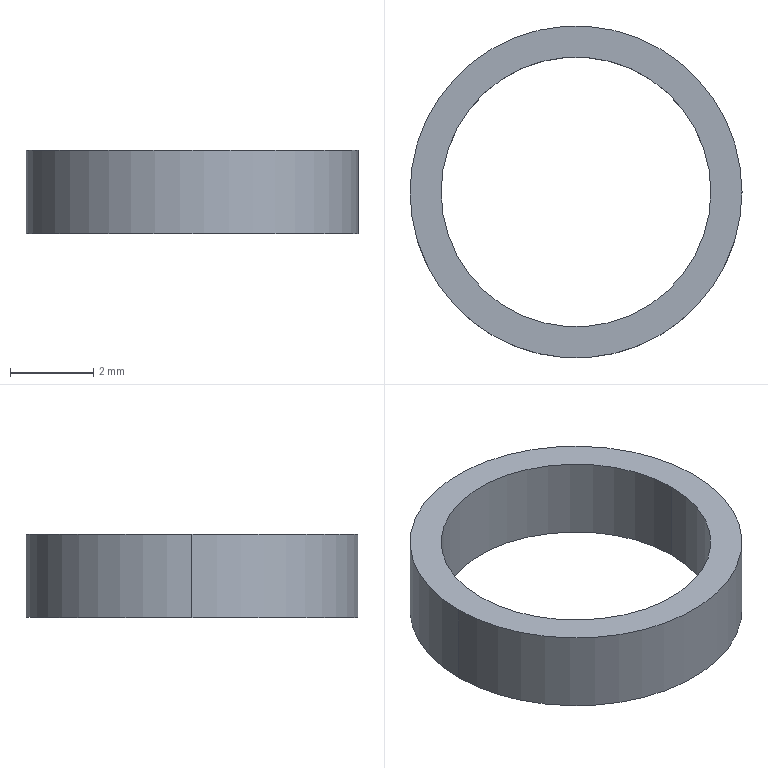Part | STEP file | 02-16 washer | 1 solid | 6 faces | box 8 x 8 x 2 mm | volume 34.165 mm3 | cylinder 4 | plane 2 | commonest cylinder face diameters 6.5 x2 8 x2
STEP:
#1=CARTESIAN_POINT('',(-3.25,0.,2.));
#2=VERTEX_POINT('',#1);
#3=CARTESIAN_POINT('',(3.25,0.,2.));
#4=VERTEX_POINT('',#3);
#5=CARTESIAN_POINT('',(0.,0.,2.));
#6=DIRECTION('',(0.,0.,1.));
#7=DIRECTION('',(1.,0.,0.));
#8=AXIS2_PLACEMENT_3D('',#5,#6,#7);
#9=CIRCLE('',#8,3.25);
#10=EDGE_CURVE('',#2,#4,#9,.T.);
#11=ORIENTED_EDGE('',*,*,#10,.T.);
#12=CARTESIAN_POINT('',(3.25,0.,0.));
#13=VERTEX_POINT('',#12);
#14=CARTESIAN_POINT('',(3.25,0.,2.));
#15=DIRECTION('',(0.,0.,-1.));
#16=VECTOR('',#15,1000.);
#17=LINE('',#14,#16);
#18=EDGE_CURVE('',#4,#13,#17,.T.);
#19=ORIENTED_EDGE('',*,*,#18,.T.);
#20=CARTESIAN_POINT('',(-3.25,0.,0.));
#21=VERTEX_POINT('',#20);
#22=CARTESIAN_POINT('',(0.,0.,0.));
#23=DIRECTION('',(0.,0.,1.));
#24=DIRECTION('',(1.,0.,0.));
#25=AXIS2_PLACEMENT_3D('',#22,#23,#24);
#26=CIRCLE('',#25,3.25);
#27=EDGE_CURVE('',#21,#13,#26,.T.);
#28=ORIENTED_EDGE('',*,*,#27,.F.);
#29=CARTESIAN_POINT('',(-3.25,0.,2.));
#30=DIRECTION('',(0.,0.,-1.));
#31=VECTOR('',#30,1000.);
#32=LINE('',#29,#31);
#33=EDGE_CURVE('',#2,#21,#32,.T.);
#34=ORIENTED_EDGE('',*,*,#33,.F.);
#35=EDGE_LOOP('',(#11,#19,#28,#34));
#36=FACE_OUTER_BOUND('',#35,.T.);
#37=CARTESIAN_POINT('',(0.,0.,2.));
#38=DIRECTION('',(0.,0.,-1.));
#39=DIRECTION('',(-1.,0.,0.));
#40=AXIS2_PLACEMENT_3D('',#37,#38,#39);
#41=CYLINDRICAL_SURFACE('',#40,3.25);
#42=ADVANCED_FACE('',(#36),#41,.F.);
#43=CARTESIAN_POINT('',(4.,0.,2.));
#44=VERTEX_POINT('',#43);
#45=CARTESIAN_POINT('',(-4.,0.,2.));
#46=VERTEX_POINT('',#45);
#47=CARTESIAN_POINT('',(0.,0.,2.));
#48=DIRECTION('',(0.,0.,1.));
#49=DIRECTION('',(1.,0.,0.));
#50=AXIS2_PLACEMENT_3D('',#47,#48,#49);
#51=CIRCLE('',#50,4.);
#52=EDGE_CURVE('',#44,#46,#51,.T.);
#53=ORIENTED_EDGE('',*,*,#52,.F.);
#54=CARTESIAN_POINT('',(4.,0.,0.));
#55=VERTEX_POINT('',#54);
#56=CARTESIAN_POINT('',(4.,0.,2.));
#57=DIRECTION('',(0.,0.,-1.));
#58=VECTOR('',#57,1000.);
#59=LINE('',#56,#58);
#60=EDGE_CURVE('',#44,#55,#59,.T.);
#61=ORIENTED_EDGE('',*,*,#60,.T.);
#62=CARTESIAN_POINT('',(-4.,0.,0.));
#63=VERTEX_POINT('',#62);
#64=CARTESIAN_POINT('',(0.,0.,0.));
#65=DIRECTION('',(0.,0.,1.));
#66=DIRECTION('',(1.,0.,0.));
#67=AXIS2_PLACEMENT_3D('',#64,#65,#66);
#68=CIRCLE('',#67,4.);
#69=EDGE_CURVE('',#55,#63,#68,.T.);
#70=ORIENTED_EDGE('',*,*,#69,.T.);
#71=CARTESIAN_POINT('',(-4.,0.,2.));
#72=DIRECTION('',(0.,0.,-1.));
#73=VECTOR('',#72,1000.);
#74=LINE('',#71,#73);
#75=EDGE_CURVE('',#46,#63,#74,.T.);
#76=ORIENTED_EDGE('',*,*,#75,.F.);
#77=EDGE_LOOP('',(#53,#61,#70,#76));
#78=FACE_OUTER_BOUND('',#77,.T.);
#79=CARTESIAN_POINT('',(0.,0.,2.));
#80=DIRECTION('',(0.,0.,-1.));
#81=DIRECTION('',(-1.,0.,0.));
#82=AXIS2_PLACEMENT_3D('',#79,#80,#81);
#83=CYLINDRICAL_SURFACE('',#82,4.);
#84=ADVANCED_FACE('',(#78),#83,.T.);
#85=CARTESIAN_POINT('',(0.,0.,2.));
#86=DIRECTION('',(0.,0.,1.));
#87=DIRECTION('',(1.,0.,0.));
#88=AXIS2_PLACEMENT_3D('',#85,#86,#87);
#89=CIRCLE('',#88,4.);
#90=EDGE_CURVE('',#46,#44,#89,.T.);
#91=ORIENTED_EDGE('',*,*,#90,.T.);
#92=ORIENTED_EDGE('',*,*,#52,.T.);
#93=EDGE_LOOP('',(#91,#92));
#94=FACE_OUTER_BOUND('',#93,.T.);
#95=ORIENTED_EDGE('',*,*,#10,.F.);
#96=CARTESIAN_POINT('',(0.,0.,2.));
#97=DIRECTION('',(0.,0.,1.));
#98=DIRECTION('',(1.,0.,0.));
#99=AXIS2_PLACEMENT_3D('',#96,#97,#98);
#100=CIRCLE('',#99,3.25);
#101=EDGE_CURVE('',#4,#2,#100,.T.);
#102=ORIENTED_EDGE('',*,*,#101,.F.);
#103=EDGE_LOOP('',(#95,#102));
#104=FACE_BOUND('',#103,.T.);
#105=CARTESIAN_POINT('',(0.,0.,2.));
#106=DIRECTION('',(0.,0.,1.));
#107=DIRECTION('',(1.,0.,0.));
#108=AXIS2_PLACEMENT_3D('',#105,#106,#107);
#109=PLANE('',#108);
#110=ADVANCED_FACE('',(#94,#104),#109,.T.);
#111=CARTESIAN_POINT('',(0.,0.,0.));
#112=DIRECTION('',(0.,0.,1.));
#113=DIRECTION('',(1.,0.,0.));
#114=AXIS2_PLACEMENT_3D('',#111,#112,#113);
#115=CIRCLE('',#114,4.);
#116=EDGE_CURVE('',#63,#55,#115,.T.);
#117=ORIENTED_EDGE('',*,*,#116,.F.);
#118=ORIENTED_EDGE('',*,*,#69,.F.);
#119=EDGE_LOOP('',(#117,#118));
#120=FACE_OUTER_BOUND('',#119,.T.);
#121=ORIENTED_EDGE('',*,*,#27,.T.);
#122=CARTESIAN_POINT('',(0.,0.,0.));
#123=DIRECTION('',(0.,0.,1.));
#124=DIRECTION('',(1.,0.,0.));
#125=AXIS2_PLACEMENT_3D('',#122,#123,#124);
#126=CIRCLE('',#125,3.25);
#127=EDGE_CURVE('',#13,#21,#126,.T.);
#128=ORIENTED_EDGE('',*,*,#127,.T.);
#129=EDGE_LOOP('',(#121,#128));
#130=FACE_BOUND('',#129,.T.);
#131=CARTESIAN_POINT('',(0.,0.,0.));
#132=DIRECTION('',(0.,0.,1.));
#133=DIRECTION('',(1.,0.,0.));
#134=AXIS2_PLACEMENT_3D('',#131,#132,#133);
#135=PLANE('',#134);
#136=ADVANCED_FACE('',(#120,#130),#135,.F.);
#137=ORIENTED_EDGE('',*,*,#60,.F.);
#138=ORIENTED_EDGE('',*,*,#90,.F.);
#139=ORIENTED_EDGE('',*,*,#75,.T.);
#140=ORIENTED_EDGE('',*,*,#116,.T.);
#141=EDGE_LOOP('',(#137,#138,#139,#140));
#142=FACE_OUTER_BOUND('',#141,.T.);
#143=CARTESIAN_POINT('',(0.,0.,2.));
#144=DIRECTION('',(0.,0.,-1.));
#145=DIRECTION('',(-1.,0.,0.));
#146=AXIS2_PLACEMENT_3D('',#143,#144,#145);
#147=CYLINDRICAL_SURFACE('',#146,4.);
#148=ADVANCED_FACE('',(#142),#147,.T.);
#149=ORIENTED_EDGE('',*,*,#18,.F.);
#150=ORIENTED_EDGE('',*,*,#101,.T.);
#151=ORIENTED_EDGE('',*,*,#33,.T.);
#152=ORIENTED_EDGE('',*,*,#127,.F.);
#153=EDGE_LOOP('',(#149,#150,#151,#152));
#154=FACE_OUTER_BOUND('',#153,.T.);
#155=CARTESIAN_POINT('',(0.,0.,2.));
#156=DIRECTION('',(0.,0.,-1.));
#157=DIRECTION('',(-1.,0.,0.));
#158=AXIS2_PLACEMENT_3D('',#155,#156,#157);
#159=CYLINDRICAL_SURFACE('',#158,3.25);
#160=ADVANCED_FACE('',(#154),#159,.F.);
#161=CLOSED_SHELL('',(#42,#84,#110,#136,#148,#160));
#162=MANIFOLD_SOLID_BREP('',#161);
#163=CARTESIAN_POINT('',(0.,0.,0.));
#164=DIRECTION('',(0.,0.,1.));
#165=DIRECTION('',(1.,0.,0.));
#166=AXIS2_PLACEMENT_3D('',#163,#164,#165);
#167=(LENGTH_UNIT()NAMED_UNIT(*)SI_UNIT(.MILLI.,.METRE.));
#168=UNCERTAINTY_MEASURE_WITH_UNIT(LENGTH_MEASURE(0.00001),#167,'','');
#169=(NAMED_UNIT(*)PLANE_ANGLE_UNIT()SI_UNIT($,.RADIAN.));
#170=(NAMED_UNIT(*)SI_UNIT($,.STERADIAN.)SOLID_ANGLE_UNIT());
#171=(GEOMETRIC_REPRESENTATION_CONTEXT(3)GLOBAL_UNCERTAINTY_ASSIGNED_CONTEXT((#168))GLOBAL_UNIT_ASSIGNED_CONTEXT((#167,#169,#170))REPRESENTATION_CONTEXT('',''));
#172=ADVANCED_BREP_SHAPE_REPRESENTATION('',(#162,#166),#171);